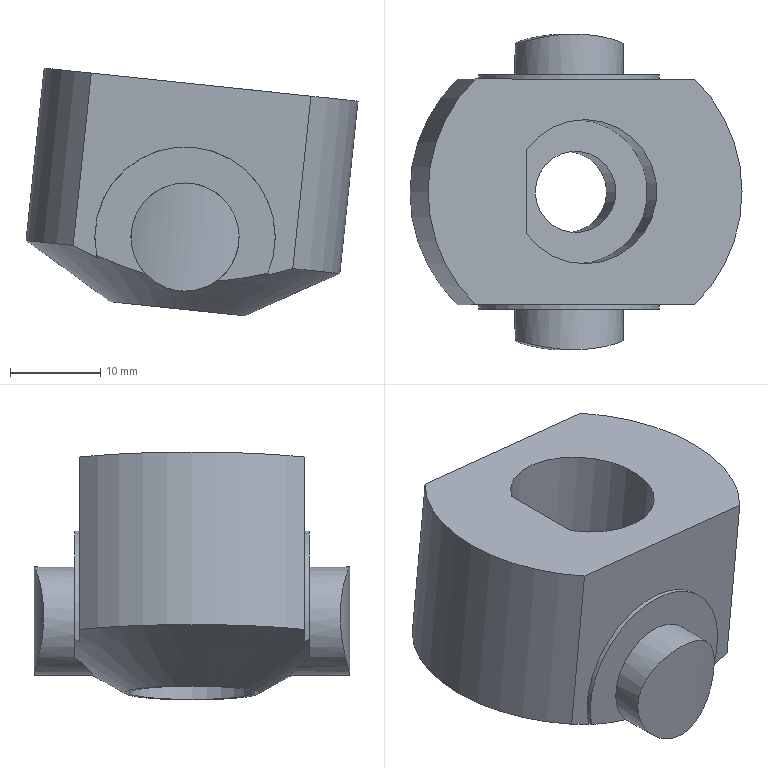Part | STEP file | P011002L001-004 | 1 solid | 21 faces | box 36.818 x 34.998 x 27.476 mm | volume 15941 mm3 | cylinder 11 | plane 9 | cone 1 | commonest cylinder face diameters 35 x4 12 x2 20 x2 9 x1 14 x1 16 x1